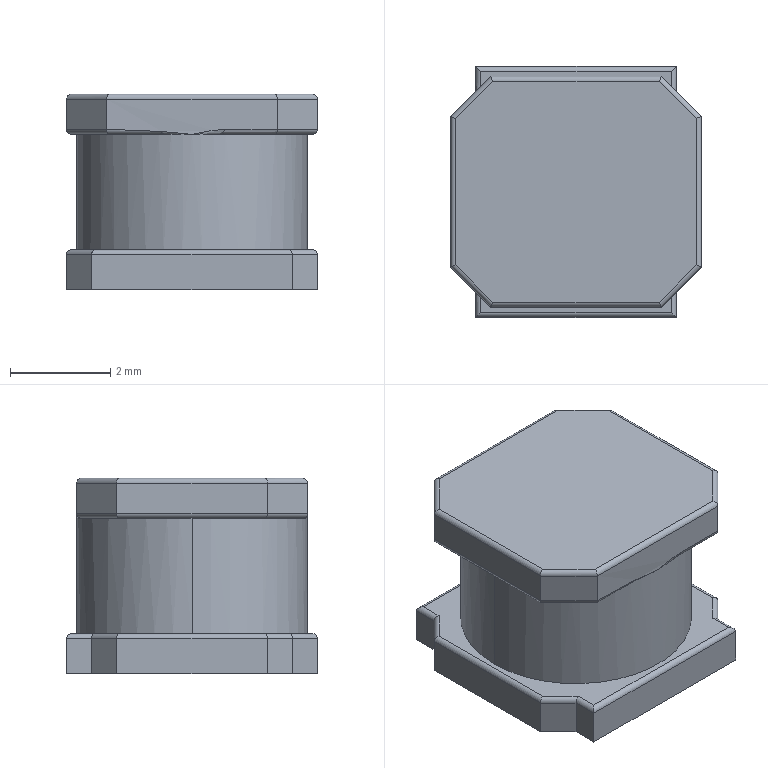Part | STEP file | RJ-USIO-V1_2-220411_267 | 1 solid | 61 faces | box 5 x 5 x 3.9 mm | volume 74.307 mm3 | cylinder 36 | plane 25 | commonest cylinder face diameters 0.2 x30 0.202 x4 4.6 x2